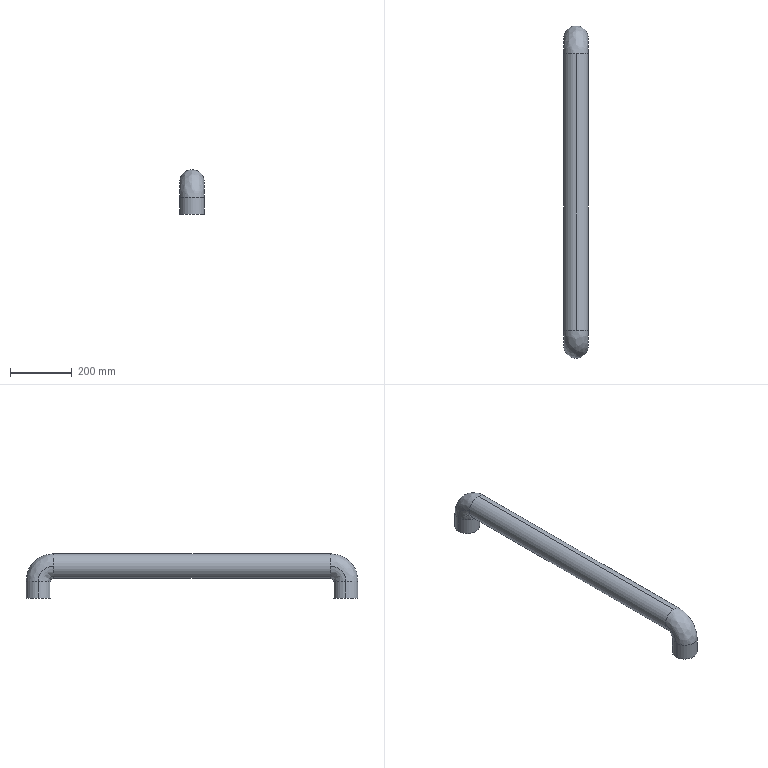Part | STEP file | Imported9 | 1 solid | 12 faces | box 80 x 1080 x 145 mm | volume 5866382 mm3 | cylinder 6 | spline 4 | plane 2 | commonest cylinder face diameters 80 x6
STEP:
#1=CARTESIAN_POINT('',(0.,0.,0.));
#2=DIRECTION('',(0.,0.,1.));
#3=DIRECTION('',(1.,0.,0.));
#4=AXIS2_PLACEMENT_3D('',#1,#2,#3);
#5=CARTESIAN_POINT('',(-920.,500.,2555.));
#6=VERTEX_POINT('',#5);
#7=CARTESIAN_POINT('',(-1000.,500.,2555.));
#8=VERTEX_POINT('',#7);
#9=CARTESIAN_POINT('',(-960.,500.,2555.));
#10=DIRECTION('',(0.,0.,1.));
#11=DIRECTION('',(-1.,0.,0.));
#12=AXIS2_PLACEMENT_3D('',#9,#10,#11);
#13=CIRCLE('',#12,40.);
#14=CARTESIAN_POINT('',(-960.,500.,2555.));
#15=DIRECTION('',(0.,0.,-1.));
#16=DIRECTION('',(-1.,0.,0.));
#17=AXIS2_PLACEMENT_3D('',#14,#15,#16);
#18=CYLINDRICAL_SURFACE('',#17,40.);
#19=CARTESIAN_POINT('',(6.283,0.));
#20=DIRECTION('',(-1.,0.));
#21=VECTOR('',#20,1.);
#22=LINE('',#19,#21);
#23=(GEOMETRIC_REPRESENTATION_CONTEXT(2)PARAMETRIC_REPRESENTATION_CONTEXT()REPRESENTATION_CONTEXT('',''));
#24=DEFINITIONAL_REPRESENTATION('',(#22),#23);
#25=PCURVE('',#18,#24);
#26=CARTESIAN_POINT('',(-1000.,500.,2555.));
#27=CARTESIAN_POINT('',(-1000.,500.,2584.289));
#28=CARTESIAN_POINT('',(-1000.,479.289,2605.));
#29=CARTESIAN_POINT('',(-1000.,450.,2605.));
#30=CARTESIAN_POINT('',(-1000.,580.,2555.));
#31=CARTESIAN_POINT('',(-1000.,580.,2631.152));
#32=CARTESIAN_POINT('',(-1000.,526.152,2685.));
#33=CARTESIAN_POINT('',(-1000.,450.,2685.));
#34=CARTESIAN_POINT('',(-920.,580.,2555.));
#35=CARTESIAN_POINT('',(-920.,580.,2631.152));
#36=CARTESIAN_POINT('',(-920.,526.152,2685.));
#37=CARTESIAN_POINT('',(-920.,450.,2685.));
#38=CARTESIAN_POINT('',(-920.,500.,2555.));
#39=CARTESIAN_POINT('',(-920.,500.,2584.289));
#40=CARTESIAN_POINT('',(-920.,479.289,2605.));
#41=CARTESIAN_POINT('',(-920.,450.,2605.));
#42=(BOUNDED_SURFACE()B_SPLINE_SURFACE(3,3,((#26,#27,#28,#29),(#30,#31,#32,#33),(#34,#35,#36,#37),(#38,#39,#40,#41)),.UNSPECIFIED.,.F.,.F.,.F.)B_SPLINE_SURFACE_WITH_KNOTS((4,4),(4,4),(0.,1.),(0.,1.),.PIECEWISE_BEZIER_KNOTS.)GEOMETRIC_REPRESENTATION_ITEM()RATIONAL_B_SPLINE_SURFACE(((1.,0.8047,0.8047,1.),(0.3333,0.2682,0.2682,0.3333),(0.3333,0.2682,0.2682,0.3333),(1.,0.8047,0.8047,1.)))REPRESENTATION_ITEM('')SURFACE());
#43=CARTESIAN_POINT('',(1.,0.));
#44=CARTESIAN_POINT('',(0.9763,0.));
#45=CARTESIAN_POINT('',(0.9319,0.));
#46=CARTESIAN_POINT('',(0.8733,0.));
#47=CARTESIAN_POINT('',(0.8206,0.));
#48=CARTESIAN_POINT('',(0.7724,0.));
#49=CARTESIAN_POINT('',(0.7279,0.));
#50=CARTESIAN_POINT('',(0.6861,0.));
#51=CARTESIAN_POINT('',(0.6465,0.));
#52=CARTESIAN_POINT('',(0.6086,0.));
#53=CARTESIAN_POINT('',(0.5718,0.));
#54=CARTESIAN_POINT('',(0.5357,0.));
#55=CARTESIAN_POINT('',(0.5,0.));
#56=CARTESIAN_POINT('',(0.4643,0.));
#57=CARTESIAN_POINT('',(0.4282,0.));
#58=CARTESIAN_POINT('',(0.3914,0.));
#59=CARTESIAN_POINT('',(0.3535,0.));
#60=CARTESIAN_POINT('',(0.3139,0.));
#61=CARTESIAN_POINT('',(0.2721,0.));
#62=CARTESIAN_POINT('',(0.2276,0.));
#63=CARTESIAN_POINT('',(0.1794,0.));
#64=CARTESIAN_POINT('',(0.1267,0.));
#65=CARTESIAN_POINT('',(0.06805,0.));
#66=CARTESIAN_POINT('',(0.02375,0.));
#67=CARTESIAN_POINT('',(0.,0.));
#68=B_SPLINE_CURVE_WITH_KNOTS('',3,(#43,#44,#45,#46,#47,#48,#49,#50,#51,#52,#53,#54,#55,#56,#57,#58,#59,#60,#61,#62,#63,#64,#65,#66,#67),.UNSPECIFIED.,.F.,.F.,(4,1,1,1,1,1,1,1,1,1,1,1,1,1,1,1,1,1,1,1,1,1,4),(3.142,3.284,3.427,3.57,3.713,3.856,3.998,4.141,4.284,4.427,4.57,4.712,4.855,4.998,5.141,5.284,5.426,5.569,5.712,5.855,5.998,6.14,6.283),.QUASI_UNIFORM_KNOTS.);
#69=(GEOMETRIC_REPRESENTATION_CONTEXT(2)PARAMETRIC_REPRESENTATION_CONTEXT()REPRESENTATION_CONTEXT('',''));
#70=DEFINITIONAL_REPRESENTATION('',(#68),#69);
#71=PCURVE('',#42,#70);
#72=SURFACE_CURVE('',#13,(#25,#71),.PCURVE_S1.);
#73=EDGE_CURVE('',#6,#8,#72,.T.);
#74=ORIENTED_EDGE('',*,*,#73,.F.);
#75=CARTESIAN_POINT('',(-920.,500.,2500.));
#76=VERTEX_POINT('',#75);
#77=CARTESIAN_POINT('',(-920.,500.,2555.));
#78=DIRECTION('',(0.,0.,-1.));
#79=VECTOR('',#78,1.);
#80=LINE('',#77,#79);
#81=CARTESIAN_POINT('',(3.142,0.));
#82=DIRECTION('',(0.,1.));
#83=VECTOR('',#82,1.);
#84=LINE('',#81,#83);
#85=(GEOMETRIC_REPRESENTATION_CONTEXT(2)PARAMETRIC_REPRESENTATION_CONTEXT()REPRESENTATION_CONTEXT('',''));
#86=DEFINITIONAL_REPRESENTATION('',(#84),#85);
#87=PCURVE('',#18,#86);
#88=CARTESIAN_POINT('',(-960.,500.,2555.));
#89=DIRECTION('',(0.,0.,-1.));
#90=DIRECTION('',(-1.,0.,0.));
#91=AXIS2_PLACEMENT_3D('',#88,#89,#90);
#92=CYLINDRICAL_SURFACE('',#91,40.);
#93=CARTESIAN_POINT('',(3.142,0.));
#94=DIRECTION('',(0.,1.));
#95=VECTOR('',#94,1.);
#96=LINE('',#93,#95);
#97=(GEOMETRIC_REPRESENTATION_CONTEXT(2)PARAMETRIC_REPRESENTATION_CONTEXT()REPRESENTATION_CONTEXT('',''));
#98=DEFINITIONAL_REPRESENTATION('',(#96),#97);
#99=PCURVE('',#92,#98);
#100=SURFACE_CURVE('',#80,(#87,#99),.PCURVE_S1.);
#101=EDGE_CURVE('',#6,#76,#100,.T.);
#102=ORIENTED_EDGE('',*,*,#101,.T.);
#103=CARTESIAN_POINT('',(-1000.,500.,2500.));
#104=VERTEX_POINT('',#103);
#105=CARTESIAN_POINT('',(-960.,500.,2500.));
#106=DIRECTION('',(0.,0.,-1.));
#107=DIRECTION('',(-1.,0.,0.));
#108=AXIS2_PLACEMENT_3D('',#105,#106,#107);
#109=CIRCLE('',#108,40.);
#110=CARTESIAN_POINT('',(0.,55.));
#111=DIRECTION('',(1.,0.));
#112=VECTOR('',#111,1.);
#113=LINE('',#110,#112);
#114=(GEOMETRIC_REPRESENTATION_CONTEXT(2)PARAMETRIC_REPRESENTATION_CONTEXT()REPRESENTATION_CONTEXT('',''));
#115=DEFINITIONAL_REPRESENTATION('',(#113),#114);
#116=PCURVE('',#18,#115);
#117=CARTESIAN_POINT('',(0.,0.,2500.));
#118=DIRECTION('',(0.,0.,-1.));
#119=DIRECTION('',(-1.,0.,0.));
#120=AXIS2_PLACEMENT_3D('',#117,#118,#119);
#121=PLANE('',#120);
#122=CARTESIAN_POINT('',(960.,500.));
#123=DIRECTION('',(1.,0.));
#124=AXIS2_PLACEMENT_2D('',#122,#123);
#125=CIRCLE('',#124,40.);
#126=(GEOMETRIC_REPRESENTATION_CONTEXT(2)PARAMETRIC_REPRESENTATION_CONTEXT()REPRESENTATION_CONTEXT('',''));
#127=DEFINITIONAL_REPRESENTATION('',(#125),#126);
#128=PCURVE('',#121,#127);
#129=SURFACE_CURVE('',#109,(#116,#128),.PCURVE_S1.);
#130=EDGE_CURVE('',#104,#76,#129,.T.);
#131=ORIENTED_EDGE('',*,*,#130,.F.);
#132=CARTESIAN_POINT('',(-1000.,500.,2555.));
#133=DIRECTION('',(0.,0.,-1.));
#134=VECTOR('',#133,1.);
#135=LINE('',#132,#134);
#136=CARTESIAN_POINT('',(0.,0.));
#137=DIRECTION('',(0.,1.));
#138=VECTOR('',#137,1.);
#139=LINE('',#136,#138);
#140=(GEOMETRIC_REPRESENTATION_CONTEXT(2)PARAMETRIC_REPRESENTATION_CONTEXT()REPRESENTATION_CONTEXT('',''));
#141=DEFINITIONAL_REPRESENTATION('',(#139),#140);
#142=PCURVE('',#18,#141);
#143=CARTESIAN_POINT('',(6.283,0.));
#144=DIRECTION('',(0.,1.));
#145=VECTOR('',#144,1.);
#146=LINE('',#143,#145);
#147=(GEOMETRIC_REPRESENTATION_CONTEXT(2)PARAMETRIC_REPRESENTATION_CONTEXT()REPRESENTATION_CONTEXT('',''));
#148=DEFINITIONAL_REPRESENTATION('',(#146),#147);
#149=PCURVE('',#92,#148);
#150=SURFACE_CURVE('',#135,(#142,#149),.PCURVE_S1.);
#151=EDGE_CURVE('',#8,#104,#150,.T.);
#152=ORIENTED_EDGE('',*,*,#151,.F.);
#153=EDGE_LOOP('',(#74,#102,#131,#152));
#154=FACE_BOUND('',#153,.T.);
#155=ADVANCED_FACE('',(#154),#18,.T.);
#156=CARTESIAN_POINT('',(-920.,450.,2605.));
#157=VERTEX_POINT('',#156);
#158=CARTESIAN_POINT('',(-960.,450.,2645.));
#159=VERTEX_POINT('',#158);
#160=CARTESIAN_POINT('',(-960.,450.,2605.));
#161=DIRECTION('',(0.,-1.,0.));
#162=DIRECTION('',(0.,0.,-1.));
#163=AXIS2_PLACEMENT_3D('',#160,#161,#162);
#164=CIRCLE('',#163,40.);
#165=CARTESIAN_POINT('',(-960.,450.,2605.));
#166=DIRECTION('',(0.,-1.,0.));
#167=DIRECTION('',(0.,0.,-1.));
#168=AXIS2_PLACEMENT_3D('',#165,#166,#167);
#169=CYLINDRICAL_SURFACE('',#168,40.);
#170=CARTESIAN_POINT('',(0.,0.));
#171=DIRECTION('',(1.,0.));
#172=VECTOR('',#171,1.);
#173=LINE('',#170,#172);
#174=(GEOMETRIC_REPRESENTATION_CONTEXT(2)PARAMETRIC_REPRESENTATION_CONTEXT()REPRESENTATION_CONTEXT('',''));
#175=DEFINITIONAL_REPRESENTATION('',(#173),#174);
#176=PCURVE('',#169,#175);
#177=CARTESIAN_POINT('',(1.,1.));
#178=CARTESIAN_POINT('',(0.9881,1.));
#179=CARTESIAN_POINT('',(0.9651,1.));
#180=CARTESIAN_POINT('',(0.9329,1.));
#181=CARTESIAN_POINT('',(0.9026,1.));
#182=CARTESIAN_POINT('',(0.874,1.));
#183=CARTESIAN_POINT('',(0.8469,1.));
#184=CARTESIAN_POINT('',(0.8211,1.));
#185=CARTESIAN_POINT('',(0.7965,1.));
#186=CARTESIAN_POINT('',(0.7729,1.));
#187=CARTESIAN_POINT('',(0.7501,1.));
#188=CARTESIAN_POINT('',(0.7282,1.));
#189=CARTESIAN_POINT('',(0.707,1.));
#190=CARTESIAN_POINT('',(0.6864,1.));
#191=CARTESIAN_POINT('',(0.6663,1.));
#192=CARTESIAN_POINT('',(0.6467,1.));
#193=CARTESIAN_POINT('',(0.6276,1.));
#194=CARTESIAN_POINT('',(0.6087,1.));
#195=CARTESIAN_POINT('',(0.5902,1.));
#196=CARTESIAN_POINT('',(0.5719,1.));
#197=CARTESIAN_POINT('',(0.5537,1.));
#198=CARTESIAN_POINT('',(0.5357,1.));
#199=CARTESIAN_POINT('',(0.5178,1.));
#200=CARTESIAN_POINT('',(0.506,1.));
#201=CARTESIAN_POINT('',(0.5,1.));
#202=B_SPLINE_CURVE_WITH_KNOTS('',3,(#177,#178,#179,#180,#181,#182,#183,#184,#185,#186,#187,#188,#189,#190,#191,#192,#193,#194,#195,#196,#197,#198,#199,#200,#201),.UNSPECIFIED.,.F.,.F.,(4,1,1,1,1,1,1,1,1,1,1,1,1,1,1,1,1,1,1,1,1,1,4),(1.571,1.642,1.714,1.785,1.856,1.928,1.999,2.071,2.142,2.213,2.285,2.356,2.428,2.499,2.57,2.642,2.713,2.785,2.856,2.927,2.999,3.07,3.142),.QUASI_UNIFORM_KNOTS.);
#203=(GEOMETRIC_REPRESENTATION_CONTEXT(2)PARAMETRIC_REPRESENTATION_CONTEXT()REPRESENTATION_CONTEXT('',''));
#204=DEFINITIONAL_REPRESENTATION('',(#202),#203);
#205=PCURVE('',#42,#204);
#206=SURFACE_CURVE('',#164,(#176,#205),.PCURVE_S1.);
#207=EDGE_CURVE('',#157,#159,#206,.T.);
#208=ORIENTED_EDGE('',*,*,#207,.T.);
#209=CARTESIAN_POINT('',(-960.,-450.,2645.));
#210=VERTEX_POINT('',#209);
#211=CARTESIAN_POINT('',(-960.,450.,2645.));
#212=DIRECTION('',(0.,-1.,0.));
#213=VECTOR('',#212,1.);
#214=LINE('',#211,#213);
#215=CARTESIAN_POINT('',(3.142,0.));
#216=DIRECTION('',(0.,1.));
#217=VECTOR('',#216,1.);
#218=LINE('',#215,#217);
#219=(GEOMETRIC_REPRESENTATION_CONTEXT(2)PARAMETRIC_REPRESENTATION_CONTEXT()REPRESENTATION_CONTEXT('',''));
#220=DEFINITIONAL_REPRESENTATION('',(#218),#219);
#221=PCURVE('',#169,#220);
#222=CARTESIAN_POINT('',(-960.,450.,2605.));
#223=DIRECTION('',(0.,-1.,0.));
#224=DIRECTION('',(0.,0.,-1.));
#225=AXIS2_PLACEMENT_3D('',#222,#223,#224);
#226=CYLINDRICAL_SURFACE('',#225,40.);
#227=CARTESIAN_POINT('',(3.142,0.));
#228=DIRECTION('',(0.,1.));
#229=VECTOR('',#228,1.);
#230=LINE('',#227,#229);
#231=(GEOMETRIC_REPRESENTATION_CONTEXT(2)PARAMETRIC_REPRESENTATION_CONTEXT()REPRESENTATION_CONTEXT('',''));
#232=DEFINITIONAL_REPRESENTATION('',(#230),#231);
#233=PCURVE('',#226,#232);
#234=SURFACE_CURVE('',#214,(#221,#233),.PCURVE_S1.);
#235=EDGE_CURVE('',#159,#210,#234,.T.);
#236=ORIENTED_EDGE('',*,*,#235,.T.);
#237=CARTESIAN_POINT('',(-920.,-450.,2605.));
#238=VERTEX_POINT('',#237);
#239=CARTESIAN_POINT('',(-960.,-450.,2605.));
#240=DIRECTION('',(0.,-1.,0.));
#241=DIRECTION('',(1.,0.,0.));
#242=AXIS2_PLACEMENT_3D('',#239,#240,#241);
#243=CIRCLE('',#242,40.);
#244=CARTESIAN_POINT('',(1.571,900.));
#245=DIRECTION('',(1.,0.));
#246=VECTOR('',#245,1.);
#247=LINE('',#244,#246);
#248=(GEOMETRIC_REPRESENTATION_CONTEXT(2)PARAMETRIC_REPRESENTATION_CONTEXT()REPRESENTATION_CONTEXT('',''));
#249=DEFINITIONAL_REPRESENTATION('',(#247),#248);
#250=PCURVE('',#169,#249);
#251=CARTESIAN_POINT('',(-1000.,-450.,2605.));
#252=CARTESIAN_POINT('',(-1000.,-479.289,2605.));
#253=CARTESIAN_POINT('',(-1000.,-500.,2584.289));
#254=CARTESIAN_POINT('',(-1000.,-500.,2555.));
#255=CARTESIAN_POINT('',(-1000.,-450.,2685.));
#256=CARTESIAN_POINT('',(-1000.,-526.152,2685.));
#257=CARTESIAN_POINT('',(-1000.,-580.,2631.152));
#258=CARTESIAN_POINT('',(-1000.,-580.,2555.));
#259=CARTESIAN_POINT('',(-920.,-450.,2685.));
#260=CARTESIAN_POINT('',(-920.,-526.152,2685.));
#261=CARTESIAN_POINT('',(-920.,-580.,2631.152));
#262=CARTESIAN_POINT('',(-920.,-580.,2555.));
#263=CARTESIAN_POINT('',(-920.,-450.,2605.));
#264=CARTESIAN_POINT('',(-920.,-479.289,2605.));
#265=CARTESIAN_POINT('',(-920.,-500.,2584.289));
#266=CARTESIAN_POINT('',(-920.,-500.,2555.));
#267=(BOUNDED_SURFACE()B_SPLINE_SURFACE(3,3,((#251,#252,#253,#254),(#255,#256,#257,#258),(#259,#260,#261,#262),(#263,#264,#265,#266)),.UNSPECIFIED.,.F.,.F.,.F.)B_SPLINE_SURFACE_WITH_KNOTS((4,4),(4,4),(0.,1.),(0.,1.),.PIECEWISE_BEZIER_KNOTS.)GEOMETRIC_REPRESENTATION_ITEM()RATIONAL_B_SPLINE_SURFACE(((1.,0.8047,0.8047,1.),(0.3333,0.2682,0.2682,0.3333),(0.3333,0.2682,0.2682,0.3333),(1.,0.8047,0.8047,1.)))REPRESENTATION_ITEM('')SURFACE());
#268=CARTESIAN_POINT('',(1.,0.));
#269=CARTESIAN_POINT('',(0.9881,0.));
#270=CARTESIAN_POINT('',(0.9651,0.));
#271=CARTESIAN_POINT('',(0.9329,0.));
#272=CARTESIAN_POINT('',(0.9026,0.));
#273=CARTESIAN_POINT('',(0.874,0.));
#274=CARTESIAN_POINT('',(0.8469,0.));
#275=CARTESIAN_POINT('',(0.8211,0.));
#276=CARTESIAN_POINT('',(0.7965,0.));
#277=CARTESIAN_POINT('',(0.7729,0.));
#278=CARTESIAN_POINT('',(0.7501,0.));
#279=CARTESIAN_POINT('',(0.7282,0.));
#280=CARTESIAN_POINT('',(0.707,0.));
#281=CARTESIAN_POINT('',(0.6864,0.));
#282=CARTESIAN_POINT('',(0.6663,0.));
#283=CARTESIAN_POINT('',(0.6467,0.));
#284=CARTESIAN_POINT('',(0.6276,0.));
#285=CARTESIAN_POINT('',(0.6087,0.));
#286=CARTESIAN_POINT('',(0.5902,0.));
#287=CARTESIAN_POINT('',(0.5719,0.));
#288=CARTESIAN_POINT('',(0.5537,0.));
#289=CARTESIAN_POINT('',(0.5357,0.));
#290=CARTESIAN_POINT('',(0.5178,0.));
#291=CARTESIAN_POINT('',(0.506,0.));
#292=CARTESIAN_POINT('',(0.5,0.));
#293=B_SPLINE_CURVE_WITH_KNOTS('',3,(#268,#269,#270,#271,#272,#273,#274,#275,#276,#277,#278,#279,#280,#281,#282,#283,#284,#285,#286,#287,#288,#289,#290,#291,#292),.UNSPECIFIED.,.F.,.F.,(4,1,1,1,1,1,1,1,1,1,1,1,1,1,1,1,1,1,1,1,1,1,4),(0.,0.0714,0.1428,0.2142,0.2856,0.357,0.4284,0.4998,0.5712,0.6426,0.714,0.7854,0.8568,0.9282,0.9996,1.071,1.142,1.214,1.285,1.357,1.428,1.499,1.571),.QUASI_UNIFORM_KNOTS.);
#294=(GEOMETRIC_REPRESENTATION_CONTEXT(2)PARAMETRIC_REPRESENTATION_CONTEXT()REPRESENTATION_CONTEXT('',''));
#295=DEFINITIONAL_REPRESENTATION('',(#293),#294);
#296=PCURVE('',#267,#295);
#297=SURFACE_CURVE('',#243,(#250,#296),.PCURVE_S1.);
#298=EDGE_CURVE('',#238,#210,#297,.T.);
#299=ORIENTED_EDGE('',*,*,#298,.F.);
#300=CARTESIAN_POINT('',(-960.,-450.,2565.));
#301=VERTEX_POINT('',#300);
#302=CARTESIAN_POINT('',(-960.,-450.,2605.));
#303=DIRECTION('',(0.,-1.,0.));
#304=DIRECTION('',(-1.,0.,0.));
#305=AXIS2_PLACEMENT_3D('',#302,#303,#304);
#306=CIRCLE('',#305,40.);
#307=CARTESIAN_POINT('',(-1.571,900.));
#308=DIRECTION('',(1.,0.));
#309=VECTOR('',#308,1.);
#310=LINE('',#307,#309);
#311=(GEOMETRIC_REPRESENTATION_CONTEXT(2)PARAMETRIC_REPRESENTATION_CONTEXT()REPRESENTATION_CONTEXT('',''));
#312=DEFINITIONAL_REPRESENTATION('',(#310),#311);
#313=PCURVE('',#169,#312);
#314=CARTESIAN_POINT('',(-920.,-450.,2605.));
#315=CARTESIAN_POINT('',(-920.,-479.289,2605.));
#316=CARTESIAN_POINT('',(-920.,-500.,2584.289));
#317=CARTESIAN_POINT('',(-920.,-500.,2555.));
#318=CARTESIAN_POINT('',(-920.,-450.,2525.));
#319=CARTESIAN_POINT('',(-920.,-432.426,2525.));
#320=CARTESIAN_POINT('',(-920.,-420.,2537.426));
#321=CARTESIAN_POINT('',(-920.,-420.,2555.));
#322=CARTESIAN_POINT('',(-1000.,-450.,2525.));
#323=CARTESIAN_POINT('',(-1000.,-432.426,2525.));
#324=CARTESIAN_POINT('',(-1000.,-420.,2537.426));
#325=CARTESIAN_POINT('',(-1000.,-420.,2555.));
#326=CARTESIAN_POINT('',(-1000.,-450.,2605.));
#327=CARTESIAN_POINT('',(-1000.,-479.289,2605.));
#328=CARTESIAN_POINT('',(-1000.,-500.,2584.289));
#329=CARTESIAN_POINT('',(-1000.,-500.,2555.));
#330=(BOUNDED_SURFACE()B_SPLINE_SURFACE(3,3,((#314,#315,#316,#317),(#318,#319,#320,#321),(#322,#323,#324,#325),(#326,#327,#328,#329)),.UNSPECIFIED.,.F.,.F.,.F.)B_SPLINE_SURFACE_WITH_KNOTS((4,4),(4,4),(0.,1.),(0.,1.),.PIECEWISE_BEZIER_KNOTS.)GEOMETRIC_REPRESENTATION_ITEM()RATIONAL_B_SPLINE_SURFACE(((1.,0.8047,0.8047,1.),(0.3333,0.2682,0.2682,0.3333),(0.3333,0.2682,0.2682,0.3333),(1.,0.8047,0.8047,1.)))REPRESENTATION_ITEM('')SURFACE());
#331=CARTESIAN_POINT('',(0.5,0.));
#332=CARTESIAN_POINT('',(0.494,0.));
#333=CARTESIAN_POINT('',(0.4822,0.));
#334=CARTESIAN_POINT('',(0.4643,0.));
#335=CARTESIAN_POINT('',(0.4463,0.));
#336=CARTESIAN_POINT('',(0.4281,0.));
#337=CARTESIAN_POINT('',(0.4098,0.));
#338=CARTESIAN_POINT('',(0.3913,0.));
#339=CARTESIAN_POINT('',(0.3724,0.));
#340=CARTESIAN_POINT('',(0.3533,0.));
#341=CARTESIAN_POINT('',(0.3337,0.));
#342=CARTESIAN_POINT('',(0.3136,0.));
#343=CARTESIAN_POINT('',(0.293,0.));
#344=CARTESIAN_POINT('',(0.2718,0.));
#345=CARTESIAN_POINT('',(0.2499,0.));
#346=CARTESIAN_POINT('',(0.2271,0.));
#347=CARTESIAN_POINT('',(0.2035,0.));
#348=CARTESIAN_POINT('',(0.1789,0.));
#349=CARTESIAN_POINT('',(0.1531,0.));
#350=CARTESIAN_POINT('',(0.126,0.));
#351=CARTESIAN_POINT('',(0.09736,0.));
#352=CARTESIAN_POINT('',(0.06707,0.));
#353=CARTESIAN_POINT('',(0.03485,0.));
#354=CARTESIAN_POINT('',(0.0119,0.));
#355=CARTESIAN_POINT('',(0.,0.));
#356=B_SPLINE_CURVE_WITH_KNOTS('',3,(#331,#332,#333,#334,#335,#336,#337,#338,#339,#340,#341,#342,#343,#344,#345,#346,#347,#348,#349,#350,#351,#352,#353,#354,#355),.UNSPECIFIED.,.F.,.F.,(4,1,1,1,1,1,1,1,1,1,1,1,1,1,1,1,1,1,1,1,1,1,4),(1.571,1.642,1.714,1.785,1.856,1.928,1.999,2.071,2.142,2.213,2.285,2.356,2.428,2.499,2.57,2.642,2.713,2.785,2.856,2.927,2.999,3.07,3.142),.QUASI_UNIFORM_KNOTS.);
#357=(GEOMETRIC_REPRESENTATION_CONTEXT(2)PARAMETRIC_REPRESENTATION_CONTEXT()REPRESENTATION_CONTEXT('',''));
#358=DEFINITIONAL_REPRESENTATION('',(#356),#357);
#359=PCURVE('',#330,#358);
#360=SURFACE_CURVE('',#306,(#313,#359),.PCURVE_S1.);
#361=EDGE_CURVE('',#301,#238,#360,.T.);
#362=ORIENTED_EDGE('',*,*,#361,.F.);
#363=CARTESIAN_POINT('',(-960.,450.,2565.));
#364=VERTEX_POINT('',#363);
#365=CARTESIAN_POINT('',(-960.,450.,2565.));
#366=DIRECTION('',(0.,-1.,0.));
#367=VECTOR('',#366,1.);
#368=LINE('',#365,#367);
#369=CARTESIAN_POINT('',(0.,0.));
#370=DIRECTION('',(0.,1.));
#371=VECTOR('',#370,1.);
#372=LINE('',#369,#371);
#373=(GEOMETRIC_REPRESENTATION_CONTEXT(2)PARAMETRIC_REPRESENTATION_CONTEXT()REPRESENTATION_CONTEXT('',''));
#374=DEFINITIONAL_REPRESENTATION('',(#372),#373);
#375=PCURVE('',#169,#374);
#376=CARTESIAN_POINT('',(6.283,0.));
#377=DIRECTION('',(0.,1.));
#378=VECTOR('',#377,1.);
#379=LINE('',#376,#378);
#380=(GEOMETRIC_REPRESENTATION_CONTEXT(2)PARAMETRIC_REPRESENTATION_CONTEXT()REPRESENTATION_CONTEXT('',''));
#381=DEFINITIONAL_REPRESENTATION('',(#379),#380);
#382=PCURVE('',#226,#381);
#383=SURFACE_CURVE('',#368,(#375,#382),.PCURVE_S1.);
#384=EDGE_CURVE('',#364,#301,#383,.T.);
#385=ORIENTED_EDGE('',*,*,#384,.F.);
#386=CARTESIAN_POINT('',(-960.,450.,2605.));
#387=DIRECTION('',(0.,-1.,0.));
#388=DIRECTION('',(0.,0.,-1.));
#389=AXIS2_PLACEMENT_3D('',#386,#387,#388);
#390=CIRCLE('',#389,40.);
#391=CARTESIAN_POINT('',(0.,0.));
#392=DIRECTION('',(1.,0.));
#393=VECTOR('',#392,1.);
#394=LINE('',#391,#393);
#395=(GEOMETRIC_REPRESENTATION_CONTEXT(2)PARAMETRIC_REPRESENTATION_CONTEXT()REPRESENTATION_CONTEXT('',''));
#396=DEFINITIONAL_REPRESENTATION('',(#394),#395);
#397=PCURVE('',#169,#396);
#398=CARTESIAN_POINT('',(-920.,500.,2555.));
#399=CARTESIAN_POINT('',(-920.,500.,2584.289));
#400=CARTESIAN_POINT('',(-920.,479.289,2605.));
#401=CARTESIAN_POINT('',(-920.,450.,2605.));
#402=CARTESIAN_POINT('',(-920.,420.,2555.));
#403=CARTESIAN_POINT('',(-920.,420.,2537.426));
#404=CARTESIAN_POINT('',(-920.,432.426,2525.));
#405=CARTESIAN_POINT('',(-920.,450.,2525.));
#406=CARTESIAN_POINT('',(-1000.,420.,2555.));
#407=CARTESIAN_POINT('',(-1000.,420.,2537.426));
#408=CARTESIAN_POINT('',(-1000.,432.426,2525.));
#409=CARTESIAN_POINT('',(-1000.,450.,2525.));
#410=CARTESIAN_POINT('',(-1000.,500.,2555.));
#411=CARTESIAN_POINT('',(-1000.,500.,2584.289));
#412=CARTESIAN_POINT('',(-1000.,479.289,2605.));
#413=CARTESIAN_POINT('',(-1000.,450.,2605.));
#414=(BOUNDED_SURFACE()B_SPLINE_SURFACE(3,3,((#398,#399,#400,#401),(#402,#403,#404,#405),(#406,#407,#408,#409),(#410,#411,#412,#413)),.UNSPECIFIED.,.F.,.F.,.F.)B_SPLINE_SURFACE_WITH_KNOTS((4,4),(4,4),(0.,1.),(0.,1.),.PIECEWISE_BEZIER_KNOTS.)GEOMETRIC_REPRESENTATION_ITEM()RATIONAL_B_SPLINE_SURFACE(((1.,0.8047,0.8047,1.),(0.3333,0.2682,0.2682,0.3333),(0.3333,0.2682,0.2682,0.3333),(1.,0.8047,0.8047,1.)))REPRESENTATION_ITEM('')SURFACE());
#415=CARTESIAN_POINT('',(0.5,1.));
#416=CARTESIAN_POINT('',(0.494,1.));
#417=CARTESIAN_POINT('',(0.4822,1.));
#418=CARTESIAN_POINT('',(0.4643,1.));
#419=CARTESIAN_POINT('',(0.4463,1.));
#420=CARTESIAN_POINT('',(0.4281,1.));
#421=CARTESIAN_POINT('',(0.4098,1.));
#422=CARTESIAN_POINT('',(0.3913,1.));
#423=CARTESIAN_POINT('',(0.3724,1.));
#424=CARTESIAN_POINT('',(0.3533,1.));
#425=CARTESIAN_POINT('',(0.3337,1.));
#426=CARTESIAN_POINT('',(0.3136,1.));
#427=CARTESIAN_POINT('',(0.293,1.));
#428=CARTESIAN_POINT('',(0.2718,1.));
#429=CARTESIAN_POINT('',(0.2499,1.));
#430=CARTESIAN_POINT('',(0.2271,1.));
#431=CARTESIAN_POINT('',(0.2035,1.));
#432=CARTESIAN_POINT('',(0.1789,1.));
#433=CARTESIAN_POINT('',(0.1531,1.));
#434=CARTESIAN_POINT('',(0.126,1.));
#435=CARTESIAN_POINT('',(0.09736,1.));
#436=CARTESIAN_POINT('',(0.06707,1.));
#437=CARTESIAN_POINT('',(0.03485,1.));
#438=CARTESIAN_POINT('',(0.0119,1.));
#439=CARTESIAN_POINT('',(0.,1.));
#440=B_SPLINE_CURVE_WITH_KNOTS('',3,(#415,#416,#417,#418,#419,#420,#421,#422,#423,#424,#425,#426,#427,#428,#429,#430,#431,#432,#433,#434,#435,#436,#437,#438,#439),.UNSPECIFIED.,.F.,.F.,(4,1,1,1,1,1,1,1,1,1,1,1,1,1,1,1,1,1,1,1,1,1,4),(0.,0.0714,0.1428,0.2142,0.2856,0.357,0.4284,0.4998,0.5712,0.6426,0.714,0.7854,0.8568,0.9282,0.9996,1.071,1.142,1.214,1.285,1.357,1.428,1.499,1.571),.QUASI_UNIFORM_KNOTS.);
#441=(GEOMETRIC_REPRESENTATION_CONTEXT(2)PARAMETRIC_REPRESENTATION_CONTEXT()REPRESENTATION_CONTEXT('',''));
#442=DEFINITIONAL_REPRESENTATION('',(#440),#441);
#443=PCURVE('',#414,#442);
#444=SURFACE_CURVE('',#390,(#397,#443),.PCURVE_S1.);
#445=EDGE_CURVE('',#364,#157,#444,.T.);
#446=ORIENTED_EDGE('',*,*,#445,.T.);
#447=EDGE_LOOP('',(#208,#236,#299,#362,#385,#446));
#448=FACE_BOUND('',#447,.T.);
#449=ADVANCED_FACE('',(#448),#169,.T.);
#450=CARTESIAN_POINT('',(-1000.,-500.,2555.));
#451=VERTEX_POINT('',#450);
#452=CARTESIAN_POINT('',(-920.,-500.,2555.));
#453=VERTEX_POINT('',#452);
#454=CARTESIAN_POINT('',(-960.,-500.,2555.));
#455=DIRECTION('',(0.,0.,-1.));
#456=DIRECTION('',(0.,1.,0.));
#457=AXIS2_PLACEMENT_3D('',#454,#455,#456);
#458=CIRCLE('',#457,40.);
#459=CARTESIAN_POINT('',(-960.,-500.,2555.));
#460=DIRECTION('',(0.,0.,-1.));
#461=DIRECTION('',(-1.,0.,0.));
#462=AXIS2_PLACEMENT_3D('',#459,#460,#461);
#463=CYLINDRICAL_SURFACE('',#462,40.);
#464=CARTESIAN_POINT('',(-4.712,0.));
#465=DIRECTION('',(1.,0.));
#466=VECTOR('',#465,1.);
#467=LINE('',#464,#466);
#468=(GEOMETRIC_REPRESENTATION_CONTEXT(2)PARAMETRIC_REPRESENTATION_CONTEXT()REPRESENTATION_CONTEXT('',''));
#469=DEFINITIONAL_REPRESENTATION('',(#467),#468);
#470=PCURVE('',#463,#469);
#471=CARTESIAN_POINT('',(1.,1.));
#472=CARTESIAN_POINT('',(0.9763,1.));
#473=CARTESIAN_POINT('',(0.9319,1.));
#474=CARTESIAN_POINT('',(0.8733,1.));
#475=CARTESIAN_POINT('',(0.8206,1.));
#476=CARTESIAN_POINT('',(0.7724,1.));
#477=CARTESIAN_POINT('',(0.7279,1.));
#478=CARTESIAN_POINT('',(0.6861,1.));
#479=CARTESIAN_POINT('',(0.6465,1.));
#480=CARTESIAN_POINT('',(0.6086,1.));
#481=CARTESIAN_POINT('',(0.5718,1.));
#482=CARTESIAN_POINT('',(0.5357,1.));
#483=CARTESIAN_POINT('',(0.5,1.));
#484=CARTESIAN_POINT('',(0.4643,1.));
#485=CARTESIAN_POINT('',(0.4282,1.));
#486=CARTESIAN_POINT('',(0.3914,1.));
#487=CARTESIAN_POINT('',(0.3535,1.));
#488=CARTESIAN_POINT('',(0.3139,1.));
#489=CARTESIAN_POINT('',(0.2721,1.));
#490=CARTESIAN_POINT('',(0.2276,1.));
#491=CARTESIAN_POINT('',(0.1794,1.));
#492=CARTESIAN_POINT('',(0.1267,1.));
#493=CARTESIAN_POINT('',(0.06805,1.));
#494=CARTESIAN_POINT('',(0.02375,1.));
#495=CARTESIAN_POINT('',(0.,1.));
#496=B_SPLINE_CURVE_WITH_KNOTS('',3,(#471,#472,#473,#474,#475,#476,#477,#478,#479,#480,#481,#482,#483,#484,#485,#486,#487,#488,#489,#490,#491,#492,#493,#494,#495),.UNSPECIFIED.,.F.,.F.,(4,1,1,1,1,1,1,1,1,1,1,1,1,1,1,1,1,1,1,1,1,1,4),(4.712,4.855,4.998,5.141,5.284,5.426,5.569,5.712,5.855,5.998,6.14,6.283,6.426,6.569,6.712,6.854,6.997,7.14,7.283,7.426,7.568,7.711,7.854),.QUASI_UNIFORM_KNOTS.);
#497=(GEOMETRIC_REPRESENTATION_CONTEXT(2)PARAMETRIC_REPRESENTATION_CONTEXT()REPRESENTATION_CONTEXT('',''));
#498=DEFINITIONAL_REPRESENTATION('',(#496),#497);
#499=PCURVE('',#330,#498);
#500=SURFACE_CURVE('',#458,(#470,#499),.PCURVE_S1.);
#501=EDGE_CURVE('',#451,#453,#500,.T.);
#502=ORIENTED_EDGE('',*,*,#501,.T.);
#503=CARTESIAN_POINT('',(-920.,-500.,2500.));
#504=VERTEX_POINT('',#503);
#505=CARTESIAN_POINT('',(-920.,-500.,2555.));
#506=DIRECTION('',(0.,0.,-1.));
#507=VECTOR('',#506,1.);
#508=LINE('',#505,#507);
#509=CARTESIAN_POINT('',(3.142,0.));
#510=DIRECTION('',(0.,1.));
#511=VECTOR('',#510,1.);
#512=LINE('',#509,#511);
#513=(GEOMETRIC_REPRESENTATION_CONTEXT(2)PARAMETRIC_REPRESENTATION_CONTEXT()REPRESENTATION_CONTEXT('',''));
#514=DEFINITIONAL_REPRESENTATION('',(#512),#513);
#515=PCURVE('',#463,#514);
#516=CARTESIAN_POINT('',(-960.,-500.,2555.));
#517=DIRECTION('',(0.,0.,-1.));
#518=DIRECTION('',(-1.,0.,0.));
#519=AXIS2_PLACEMENT_3D('',#516,#517,#518);
#520=CYLINDRICAL_SURFACE('',#519,40.);
#521=CARTESIAN_POINT('',(3.142,0.));
#522=DIRECTION('',(0.,1.));
#523=VECTOR('',#522,1.);
#524=LINE('',#521,#523);
#525=(GEOMETRIC_REPRESENTATION_CONTEXT(2)PARAMETRIC_REPRESENTATION_CONTEXT()REPRESENTATION_CONTEXT('',''));
#526=DEFINITIONAL_REPRESENTATION('',(#524),#525);
#527=PCURVE('',#520,#526);
#528=SURFACE_CURVE('',#508,(#515,#527),.PCURVE_S1.);
#529=EDGE_CURVE('',#453,#504,#528,.T.);
#530=ORIENTED_EDGE('',*,*,#529,.T.);
#531=CARTESIAN_POINT('',(-1000.,-500.,2500.));
#532=VERTEX_POINT('',#531);
#533=CARTESIAN_POINT('',(-960.,-500.,2500.));
#534=DIRECTION('',(0.,0.,-1.));
#535=DIRECTION('',(-1.,0.,0.));
#536=AXIS2_PLACEMENT_3D('',#533,#534,#535);
#537=CIRCLE('',#536,40.);
#538=CARTESIAN_POINT('',(0.,55.));
#539=DIRECTION('',(1.,0.));
#540=VECTOR('',#539,1.);
#541=LINE('',#538,#540);
#542=(GEOMETRIC_REPRESENTATION_CONTEXT(2)PARAMETRIC_REPRESENTATION_CONTEXT()REPRESENTATION_CONTEXT('',''));
#543=DEFINITIONAL_REPRESENTATION('',(#541),#542);
#544=PCURVE('',#463,#543);
#545=CARTESIAN_POINT('',(0.,0.,2500.));
#546=DIRECTION('',(0.,0.,-1.));
#547=DIRECTION('',(-1.,0.,0.));
#548=AXIS2_PLACEMENT_3D('',#545,#546,#547);
#549=PLANE('',#548);
#550=CARTESIAN_POINT('',(960.,-500.));
#551=DIRECTION('',(1.,0.));
#552=AXIS2_PLACEMENT_2D('',#550,#551);
#553=CIRCLE('',#552,40.);
#554=(GEOMETRIC_REPRESENTATION_CONTEXT(2)PARAMETRIC_REPRESENTATION_CONTEXT()REPRESENTATION_CONTEXT('',''));
#555=DEFINITIONAL_REPRESENTATION('',(#553),#554);
#556=PCURVE('',#549,#555);
#557=SURFACE_CURVE('',#537,(#544,#556),.PCURVE_S1.);
#558=EDGE_CURVE('',#532,#504,#557,.T.);
#559=ORIENTED_EDGE('',*,*,#558,.F.);
#560=CARTESIAN_POINT('',(-1000.,-500.,2555.));
#561=DIRECTION('',(0.,0.,-1.));
#562=VECTOR('',#561,1.);
#563=LINE('',#560,#562);
#564=CARTESIAN_POINT('',(0.,0.));
#565=DIRECTION('',(0.,1.));
#566=VECTOR('',#565,1.);
#567=LINE('',#564,#566);
#568=(GEOMETRIC_REPRESENTATION_CONTEXT(2)PARAMETRIC_REPRESENTATION_CONTEXT()REPRESENTATION_CONTEXT('',''));
#569=DEFINITIONAL_REPRESENTATION('',(#567),#568);
#570=PCURVE('',#463,#569);
#571=CARTESIAN_POINT('',(6.283,0.));
#572=DIRECTION('',(0.,1.));
#573=VECTOR('',#572,1.);
#574=LINE('',#571,#573);
#575=(GEOMETRIC_REPRESENTATION_CONTEXT(2)PARAMETRIC_REPRESENTATION_CONTEXT()REPRESENTATION_CONTEXT('',''));
#576=DEFINITIONAL_REPRESENTATION('',(#574),#575);
#577=PCURVE('',#520,#576);
#578=SURFACE_CURVE('',#563,(#570,#577),.PCURVE_S1.);
#579=EDGE_CURVE('',#451,#532,#578,.T.);
#580=ORIENTED_EDGE('',*,*,#579,.F.);
#581=EDGE_LOOP('',(#502,#530,#559,#580));
#582=FACE_BOUND('',#581,.T.);
#583=ADVANCED_FACE('',(#582),#463,.T.);
#584=ORIENTED_EDGE('',*,*,#101,.F.);
#585=CARTESIAN_POINT('',(-960.,500.,2555.));
#586=DIRECTION('',(0.,0.,1.));
#587=DIRECTION('',(1.,0.,0.));
#588=AXIS2_PLACEMENT_3D('',#585,#586,#587);
#589=CIRCLE('',#588,40.);
#590=CARTESIAN_POINT('',(9.425,0.));
#591=DIRECTION('',(-1.,0.));
#592=VECTOR('',#591,1.);
#593=LINE('',#590,#592);
#594=(GEOMETRIC_REPRESENTATION_CONTEXT(2)PARAMETRIC_REPRESENTATION_CONTEXT()REPRESENTATION_CONTEXT('',''));
#595=DEFINITIONAL_REPRESENTATION('',(#593),#594);
#596=PCURVE('',#92,#595);
#597=CARTESIAN_POINT('',(1.,0.));
#598=CARTESIAN_POINT('',(0.9763,0.));
#599=CARTESIAN_POINT('',(0.9319,0.));
#600=CARTESIAN_POINT('',(0.8733,0.));
#601=CARTESIAN_POINT('',(0.8206,0.));
#602=CARTESIAN_POINT('',(0.7724,0.));
#603=CARTESIAN_POINT('',(0.7279,0.));
#604=CARTESIAN_POINT('',(0.6861,0.));
#605=CARTESIAN_POINT('',(0.6465,0.));
#606=CARTESIAN_POINT('',(0.6086,0.));
#607=CARTESIAN_POINT('',(0.5718,0.));
#608=CARTESIAN_POINT('',(0.5357,0.));
#609=CARTESIAN_POINT('',(0.5,0.));
#610=CARTESIAN_POINT('',(0.4643,0.));
#611=CARTESIAN_POINT('',(0.4282,0.));
#612=CARTESIAN_POINT('',(0.3914,0.));
#613=CARTESIAN_POINT('',(0.3535,0.));
#614=CARTESIAN_POINT('',(0.3139,0.));
#615=CARTESIAN_POINT('',(0.2721,0.));
#616=CARTESIAN_POINT('',(0.2276,0.));
#617=CARTESIAN_POINT('',(0.1794,0.));
#618=CARTESIAN_POINT('',(0.1267,0.));
#619=CARTESIAN_POINT('',(0.06805,0.));
#620=CARTESIAN_POINT('',(0.02375,0.));
#621=CARTESIAN_POINT('',(0.,0.));
#622=B_SPLINE_CURVE_WITH_KNOTS('',3,(#597,#598,#599,#600,#601,#602,#603,#604,#605,#606,#607,#608,#609,#610,#611,#612,#613,#614,#615,#616,#617,#618,#619,#620,#621),.UNSPECIFIED.,.F.,.F.,(4,1,1,1,1,1,1,1,1,1,1,1,1,1,1,1,1,1,1,1,1,1,4),(3.142,3.284,3.427,3.57,3.713,3.856,3.998,4.141,4.284,4.427,4.57,4.712,4.855,4.998,5.141,5.284,5.426,5.569,5.712,5.855,5.998,6.14,6.283),.QUASI_UNIFORM_KNOTS.);
#623=(GEOMETRIC_REPRESENTATION_CONTEXT(2)PARAMETRIC_REPRESENTATION_CONTEXT()REPRESENTATION_CONTEXT('',''));
#624=DEFINITIONAL_REPRESENTATION('',(#622),#623);
#625=PCURVE('',#414,#624);
#626=SURFACE_CURVE('',#589,(#596,#625),.PCURVE_S1.);
#627=EDGE_CURVE('',#8,#6,#626,.T.);
#628=ORIENTED_EDGE('',*,*,#627,.F.);
#629=ORIENTED_EDGE('',*,*,#151,.T.);
#630=CARTESIAN_POINT('',(-960.,500.,2500.));
#631=DIRECTION('',(0.,0.,-1.));
#632=DIRECTION('',(-1.,0.,0.));
#633=AXIS2_PLACEMENT_3D('',#630,#631,#632);
#634=CIRCLE('',#633,40.);
#635=CARTESIAN_POINT('',(0.,55.));
#636=DIRECTION('',(1.,0.));
#637=VECTOR('',#636,1.);
#638=LINE('',#635,#637);
#639=(GEOMETRIC_REPRESENTATION_CONTEXT(2)PARAMETRIC_REPRESENTATION_CONTEXT()REPRESENTATION_CONTEXT('',''));
#640=DEFINITIONAL_REPRESENTATION('',(#638),#639);
#641=PCURVE('',#92,#640);
#642=CARTESIAN_POINT('',(960.,500.));
#643=DIRECTION('',(1.,0.));
#644=AXIS2_PLACEMENT_2D('',#642,#643);
#645=CIRCLE('',#644,40.);
#646=(GEOMETRIC_REPRESENTATION_CONTEXT(2)PARAMETRIC_REPRESENTATION_CONTEXT()REPRESENTATION_CONTEXT('',''));
#647=DEFINITIONAL_REPRESENTATION('',(#645),#646);
#648=PCURVE('',#121,#647);
#649=SURFACE_CURVE('',#634,(#641,#648),.PCURVE_S1.);
#650=EDGE_CURVE('',#76,#104,#649,.T.);
#651=ORIENTED_EDGE('',*,*,#650,.F.);
#652=EDGE_LOOP('',(#584,#628,#629,#651));
#653=FACE_BOUND('',#652,.T.);
#654=ADVANCED_FACE('',(#653),#92,.T.);
#655=ORIENTED_EDGE('',*,*,#130,.T.);
#656=ORIENTED_EDGE('',*,*,#650,.T.);
#657=EDGE_LOOP('',(#655,#656));
#658=FACE_BOUND('',#657,.T.);
#659=ADVANCED_FACE('',(#658),#121,.T.);
#660=CARTESIAN_POINT('',(-920.,450.,2555.));
#661=DIRECTION('',(1.,0.,0.));
#662=DIRECTION('',(0.,1.,0.));
#663=AXIS2_PLACEMENT_3D('',#660,#661,#662);
#664=CIRCLE('',#663,50.);
#665=CARTESIAN_POINT('',(1.,0.));
#666=CARTESIAN_POINT('',(1.,0.01683));
#667=CARTESIAN_POINT('',(1.,0.04999));
#668=CARTESIAN_POINT('',(1.,0.09843));
#669=CARTESIAN_POINT('',(1.,0.1457));
#670=CARTESIAN_POINT('',(1.,0.192));
#671=CARTESIAN_POINT('',(1.,0.2375));
#672=CARTESIAN_POINT('',(1.,0.2823));
#673=CARTESIAN_POINT('',(1.,0.3265));
#674=CARTESIAN_POINT('',(1.,0.3703));
#675=CARTESIAN_POINT('',(1.,0.4137));
#676=CARTESIAN_POINT('',(1.,0.4569));
#677=CARTESIAN_POINT('',(1.,0.5));
#678=CARTESIAN_POINT('',(1.,0.5431));
#679=CARTESIAN_POINT('',(1.,0.5863));
#680=CARTESIAN_POINT('',(1.,0.6297));
#681=CARTESIAN_POINT('',(1.,0.6735));
#682=CARTESIAN_POINT('',(1.,0.7177));
#683=CARTESIAN_POINT('',(1.,0.7625));
#684=CARTESIAN_POINT('',(1.,0.808));
#685=CARTESIAN_POINT('',(1.,0.8543));
#686=CARTESIAN_POINT('',(1.,0.9016));
#687=CARTESIAN_POINT('',(1.,0.95));
#688=CARTESIAN_POINT('',(1.,0.9832));
#689=CARTESIAN_POINT('',(1.,1.));
#690=B_SPLINE_CURVE_WITH_KNOTS('',3,(#665,#666,#667,#668,#669,#670,#671,#672,#673,#674,#675,#676,#677,#678,#679,#680,#681,#682,#683,#684,#685,#686,#687,#688,#689),.UNSPECIFIED.,.F.,.F.,(4,1,1,1,1,1,1,1,1,1,1,1,1,1,1,1,1,1,1,1,1,1,4),(0.,0.0714,0.1428,0.2142,0.2856,0.357,0.4284,0.4998,0.5712,0.6426,0.714,0.7854,0.8568,0.9282,0.9996,1.071,1.142,1.214,1.285,1.357,1.428,1.499,1.571),.QUASI_UNIFORM_KNOTS.);
#691=(GEOMETRIC_REPRESENTATION_CONTEXT(2)PARAMETRIC_REPRESENTATION_CONTEXT()REPRESENTATION_CONTEXT('',''));
#692=DEFINITIONAL_REPRESENTATION('',(#690),#691);
#693=PCURVE('',#42,#692);
#694=CARTESIAN_POINT('',(0.,0.));
#695=CARTESIAN_POINT('',(0.,0.01683));
#696=CARTESIAN_POINT('',(0.,0.04999));
#697=CARTESIAN_POINT('',(0.,0.09843));
#698=CARTESIAN_POINT('',(0.,0.1457));
#699=CARTESIAN_POINT('',(0.,0.192));
#700=CARTESIAN_POINT('',(0.,0.2375));
#701=CARTESIAN_POINT('',(0.,0.2823));
#702=CARTESIAN_POINT('',(0.,0.3265));
#703=CARTESIAN_POINT('',(0.,0.3703));
#704=CARTESIAN_POINT('',(0.,0.4137));
#705=CARTESIAN_POINT('',(0.,0.4569));
#706=CARTESIAN_POINT('',(0.,0.5));
#707=CARTESIAN_POINT('',(0.,0.5431));
#708=CARTESIAN_POINT('',(0.,0.5863));
#709=CARTESIAN_POINT('',(0.,0.6297));
#710=CARTESIAN_POINT('',(0.,0.6735));
#711=CARTESIAN_POINT('',(0.,0.7177));
#712=CARTESIAN_POINT('',(0.,0.7625));
#713=CARTESIAN_POINT('',(0.,0.808));
#714=CARTESIAN_POINT('',(0.,0.8543));
#715=CARTESIAN_POINT('',(0.,0.9016));
#716=CARTESIAN_POINT('',(0.,0.95));
#717=CARTESIAN_POINT('',(0.,0.9832));
#718=CARTESIAN_POINT('',(0.,1.));
#719=B_SPLINE_CURVE_WITH_KNOTS('',3,(#694,#695,#696,#697,#698,#699,#700,#701,#702,#703,#704,#705,#706,#707,#708,#709,#710,#711,#712,#713,#714,#715,#716,#717,#718),.UNSPECIFIED.,.F.,.F.,(4,1,1,1,1,1,1,1,1,1,1,1,1,1,1,1,1,1,1,1,1,1,4),(0.,0.0714,0.1428,0.2142,0.2856,0.357,0.4284,0.4998,0.5712,0.6426,0.714,0.7854,0.8568,0.9282,0.9996,1.071,1.142,1.214,1.285,1.357,1.428,1.499,1.571),.QUASI_UNIFORM_KNOTS.);
#720=(GEOMETRIC_REPRESENTATION_CONTEXT(2)PARAMETRIC_REPRESENTATION_CONTEXT()REPRESENTATION_CONTEXT('',''));
#721=DEFINITIONAL_REPRESENTATION('',(#719),#720);
#722=PCURVE('',#414,#721);
#723=SURFACE_CURVE('',#664,(#693,#722),.PCURVE_S1.);
#724=EDGE_CURVE('',#6,#157,#723,.T.);
#725=ORIENTED_EDGE('',*,*,#724,.T.);
#726=ORIENTED_EDGE('',*,*,#207,.T.);
#727=CARTESIAN_POINT('',(-1000.,450.,2605.));
#728=VERTEX_POINT('',#727);
#729=CARTESIAN_POINT('',(-960.,450.,2605.));
#730=DIRECTION('',(0.,-1.,0.));
#731=DIRECTION('',(0.,0.,-1.));
#732=AXIS2_PLACEMENT_3D('',#729,#730,#731);
#733=CIRCLE('',#732,40.);
#734=CARTESIAN_POINT('',(0.5,1.));
#735=CARTESIAN_POINT('',(0.494,1.));
#736=CARTESIAN_POINT('',(0.4822,1.));
#737=CARTESIAN_POINT('',(0.4643,1.));
#738=CARTESIAN_POINT('',(0.4463,1.));
#739=CARTESIAN_POINT('',(0.4281,1.));
#740=CARTESIAN_POINT('',(0.4098,1.));
#741=CARTESIAN_POINT('',(0.3913,1.));
#742=CARTESIAN_POINT('',(0.3724,1.));
#743=CARTESIAN_POINT('',(0.3533,1.));
#744=CARTESIAN_POINT('',(0.3337,1.));
#745=CARTESIAN_POINT('',(0.3136,1.));
#746=CARTESIAN_POINT('',(0.293,1.));
#747=CARTESIAN_POINT('',(0.2718,1.));
#748=CARTESIAN_POINT('',(0.2499,1.));
#749=CARTESIAN_POINT('',(0.2271,1.));
#750=CARTESIAN_POINT('',(0.2035,1.));
#751=CARTESIAN_POINT('',(0.1789,1.));
#752=CARTESIAN_POINT('',(0.1531,1.));
#753=CARTESIAN_POINT('',(0.126,1.));
#754=CARTESIAN_POINT('',(0.09736,1.));
#755=CARTESIAN_POINT('',(0.06707,1.));
#756=CARTESIAN_POINT('',(0.03485,1.));
#757=CARTESIAN_POINT('',(0.0119,1.));
#758=CARTESIAN_POINT('',(0.,1.));
#759=B_SPLINE_CURVE_WITH_KNOTS('',3,(#734,#735,#736,#737,#738,#739,#740,#741,#742,#743,#744,#745,#746,#747,#748,#749,#750,#751,#752,#753,#754,#755,#756,#757,#758),.UNSPECIFIED.,.F.,.F.,(4,1,1,1,1,1,1,1,1,1,1,1,1,1,1,1,1,1,1,1,1,1,4),(3.142,3.213,3.284,3.356,3.427,3.499,3.57,3.641,3.713,3.784,3.856,3.927,3.998,4.07,4.141,4.213,4.284,4.355,4.427,4.498,4.57,4.641,4.712),.QUASI_UNIFORM_KNOTS.);
#760=(GEOMETRIC_REPRESENTATION_CONTEXT(2)PARAMETRIC_REPRESENTATION_CONTEXT()REPRESENTATION_CONTEXT('',''));
#761=DEFINITIONAL_REPRESENTATION('',(#759),#760);
#762=PCURVE('',#42,#761);
#763=CARTESIAN_POINT('',(0.,0.));
#764=DIRECTION('',(1.,0.));
#765=VECTOR('',#764,1.);
#766=LINE('',#763,#765);
#767=(GEOMETRIC_REPRESENTATION_CONTEXT(2)PARAMETRIC_REPRESENTATION_CONTEXT()REPRESENTATION_CONTEXT('',''));
#768=DEFINITIONAL_REPRESENTATION('',(#766),#767);
#769=PCURVE('',#226,#768);
#770=SURFACE_CURVE('',#733,(#762,#769),.PCURVE_S1.);
#771=EDGE_CURVE('',#159,#728,#770,.T.);
#772=ORIENTED_EDGE('',*,*,#771,.T.);
#773=CARTESIAN_POINT('',(-1000.,450.,2555.));
#774=DIRECTION('',(-1.,0.,0.));
#775=DIRECTION('',(0.,1.,0.));
#776=AXIS2_PLACEMENT_3D('',#773,#774,#775);
#777=CIRCLE('',#776,50.);
#778=CARTESIAN_POINT('',(0.,1.));
#779=CARTESIAN_POINT('',(0.,0.9832));
#780=CARTESIAN_POINT('',(0.,0.95));
#781=CARTESIAN_POINT('',(0.,0.9016));
#782=CARTESIAN_POINT('',(0.,0.8543));
#783=CARTESIAN_POINT('',(0.,0.808));
#784=CARTESIAN_POINT('',(0.,0.7625));
#785=CARTESIAN_POINT('',(0.,0.7177));
#786=CARTESIAN_POINT('',(0.,0.6735));
#787=CARTESIAN_POINT('',(0.,0.6297));
#788=CARTESIAN_POINT('',(0.,0.5863));
#789=CARTESIAN_POINT('',(0.,0.5431));
#790=CARTESIAN_POINT('',(0.,0.5));
#791=CARTESIAN_POINT('',(0.,0.4569));
#792=CARTESIAN_POINT('',(0.,0.4137));
#793=CARTESIAN_POINT('',(0.,0.3703));
#794=CARTESIAN_POINT('',(0.,0.3265));
#795=CARTESIAN_POINT('',(0.,0.2823));
#796=CARTESIAN_POINT('',(0.,0.2375));
#797=CARTESIAN_POINT('',(0.,0.192));
#798=CARTESIAN_POINT('',(0.,0.1457));
#799=CARTESIAN_POINT('',(0.,0.09843));
#800=CARTESIAN_POINT('',(0.,0.04999));
#801=CARTESIAN_POINT('',(0.,0.01683));
#802=CARTESIAN_POINT('',(0.,0.));
#803=B_SPLINE_CURVE_WITH_KNOTS('',3,(#778,#779,#780,#781,#782,#783,#784,#785,#786,#787,#788,#789,#790,#791,#792,#793,#794,#795,#796,#797,#798,#799,#800,#801,#802),.UNSPECIFIED.,.F.,.F.,(4,1,1,1,1,1,1,1,1,1,1,1,1,1,1,1,1,1,1,1,1,1,4),(4.712,4.784,4.855,4.927,4.998,5.069,5.141,5.212,5.284,5.355,5.426,5.498,5.569,5.641,5.712,5.783,5.855,5.926,5.998,6.069,6.14,6.212,6.283),.QUASI_UNIFORM_KNOTS.);
#804=(GEOMETRIC_REPRESENTATION_CONTEXT(2)PARAMETRIC_REPRESENTATION_CONTEXT()REPRESENTATION_CONTEXT('',''));
#805=DEFINITIONAL_REPRESENTATION('',(#803),#804);
#806=PCURVE('',#42,#805);
#807=CARTESIAN_POINT('',(1.,1.));
#808=CARTESIAN_POINT('',(1.,0.9832));
#809=CARTESIAN_POINT('',(1.,0.95));
#810=CARTESIAN_POINT('',(1.,0.9016));
#811=CARTESIAN_POINT('',(1.,0.8543));
#812=CARTESIAN_POINT('',(1.,0.808));
#813=CARTESIAN_POINT('',(1.,0.7625));
#814=CARTESIAN_POINT('',(1.,0.7177));
#815=CARTESIAN_POINT('',(1.,0.6735));
#816=CARTESIAN_POINT('',(1.,0.6297));
#817=CARTESIAN_POINT('',(1.,0.5863));
#818=CARTESIAN_POINT('',(1.,0.5431));
#819=CARTESIAN_POINT('',(1.,0.5));
#820=CARTESIAN_POINT('',(1.,0.4569));
#821=CARTESIAN_POINT('',(1.,0.4137));
#822=CARTESIAN_POINT('',(1.,0.3703));
#823=CARTESIAN_POINT('',(1.,0.3265));
#824=CARTESIAN_POINT('',(1.,0.2823));
#825=CARTESIAN_POINT('',(1.,0.2375));
#826=CARTESIAN_POINT('',(1.,0.192));
#827=CARTESIAN_POINT('',(1.,0.1457));
#828=CARTESIAN_POINT('',(1.,0.09843));
#829=CARTESIAN_POINT('',(1.,0.04999));
#830=CARTESIAN_POINT('',(1.,0.01683));
#831=CARTESIAN_POINT('',(1.,0.));
#832=B_SPLINE_CURVE_WITH_KNOTS('',3,(#807,#808,#809,#810,#811,#812,#813,#814,#815,#816,#817,#818,#819,#820,#821,#822,#823,#824,#825,#826,#827,#828,#829,#830,#831),.UNSPECIFIED.,.F.,.F.,(4,1,1,1,1,1,1,1,1,1,1,1,1,1,1,1,1,1,1,1,1,1,4),(4.712,4.784,4.855,4.927,4.998,5.069,5.141,5.212,5.284,5.355,5.426,5.498,5.569,5.641,5.712,5.783,5.855,5.926,5.998,6.069,6.14,6.212,6.283),.QUASI_UNIFORM_KNOTS.);
#833=(GEOMETRIC_REPRESENTATION_CONTEXT(2)PARAMETRIC_REPRESENTATION_CONTEXT()REPRESENTATION_CONTEXT('',''));
#834=DEFINITIONAL_REPRESENTATION('',(#832),#833);
#835=PCURVE('',#414,#834);
#836=SURFACE_CURVE('',#777,(#806,#835),.PCURVE_S1.);
#837=EDGE_CURVE('',#728,#8,#836,.T.);
#838=ORIENTED_EDGE('',*,*,#837,.T.);
#839=ORIENTED_EDGE('',*,*,#73,.F.);
#840=EDGE_LOOP('',(#725,#726,#772,#838,#839));
#841=FACE_BOUND('',#840,.F.);
#842=ADVANCED_FACE('',(#841),#42,.F.);
#843=ORIENTED_EDGE('',*,*,#837,.F.);
#844=CARTESIAN_POINT('',(-960.,450.,2605.));
#845=DIRECTION('',(0.,-1.,0.));
#846=DIRECTION('',(0.,0.,-1.));
#847=AXIS2_PLACEMENT_3D('',#844,#845,#846);
#848=CIRCLE('',#847,40.);
#849=CARTESIAN_POINT('',(1.,1.));
#850=CARTESIAN_POINT('',(0.9881,1.));
#851=CARTESIAN_POINT('',(0.9651,1.));
#852=CARTESIAN_POINT('',(0.9329,1.));
#853=CARTESIAN_POINT('',(0.9026,1.));
#854=CARTESIAN_POINT('',(0.874,1.));
#855=CARTESIAN_POINT('',(0.8469,1.));
#856=CARTESIAN_POINT('',(0.8211,1.));
#857=CARTESIAN_POINT('',(0.7965,1.));
#858=CARTESIAN_POINT('',(0.7729,1.));
#859=CARTESIAN_POINT('',(0.7501,1.));
#860=CARTESIAN_POINT('',(0.7282,1.));
#861=CARTESIAN_POINT('',(0.707,1.));
#862=CARTESIAN_POINT('',(0.6864,1.));
#863=CARTESIAN_POINT('',(0.6663,1.));
#864=CARTESIAN_POINT('',(0.6467,1.));
#865=CARTESIAN_POINT('',(0.6276,1.));
#866=CARTESIAN_POINT('',(0.6087,1.));
#867=CARTESIAN_POINT('',(0.5902,1.));
#868=CARTESIAN_POINT('',(0.5719,1.));
#869=CARTESIAN_POINT('',(0.5537,1.));
#870=CARTESIAN_POINT('',(0.5357,1.));
#871=CARTESIAN_POINT('',(0.5178,1.));
#872=CARTESIAN_POINT('',(0.506,1.));
#873=CARTESIAN_POINT('',(0.5,1.));
#874=B_SPLINE_CURVE_WITH_KNOTS('',3,(#849,#850,#851,#852,#853,#854,#855,#856,#857,#858,#859,#860,#861,#862,#863,#864,#865,#866,#867,#868,#869,#870,#871,#872,#873),.UNSPECIFIED.,.F.,.F.,(4,1,1,1,1,1,1,1,1,1,1,1,1,1,1,1,1,1,1,1,1,1,4),(4.712,4.784,4.855,4.927,4.998,5.069,5.141,5.212,5.284,5.355,5.426,5.498,5.569,5.641,5.712,5.783,5.855,5.926,5.998,6.069,6.14,6.212,6.283),.QUASI_UNIFORM_KNOTS.);
#875=(GEOMETRIC_REPRESENTATION_CONTEXT(2)PARAMETRIC_REPRESENTATION_CONTEXT()REPRESENTATION_CONTEXT('',''));
#876=DEFINITIONAL_REPRESENTATION('',(#874),#875);
#877=PCURVE('',#414,#876);
#878=CARTESIAN_POINT('',(0.,0.));
#879=DIRECTION('',(1.,0.));
#880=VECTOR('',#879,1.);
#881=LINE('',#878,#880);
#882=(GEOMETRIC_REPRESENTATION_CONTEXT(2)PARAMETRIC_REPRESENTATION_CONTEXT()REPRESENTATION_CONTEXT('',''));
#883=DEFINITIONAL_REPRESENTATION('',(#881),#882);
#884=PCURVE('',#226,#883);
#885=SURFACE_CURVE('',#848,(#877,#884),.PCURVE_S1.);
#886=EDGE_CURVE('',#728,#364,#885,.T.);
#887=ORIENTED_EDGE('',*,*,#886,.T.);
#888=ORIENTED_EDGE('',*,*,#445,.T.);
#889=ORIENTED_EDGE('',*,*,#724,.F.);
#890=ORIENTED_EDGE('',*,*,#627,.F.);
#891=EDGE_LOOP('',(#843,#887,#888,#889,#890));
#892=FACE_BOUND('',#891,.F.);
#893=ADVANCED_FACE('',(#892),#414,.F.);
#894=ORIENTED_EDGE('',*,*,#235,.F.);
#895=ORIENTED_EDGE('',*,*,#771,.T.);
#896=ORIENTED_EDGE('',*,*,#886,.T.);
#897=ORIENTED_EDGE('',*,*,#384,.T.);
#898=CARTESIAN_POINT('',(-1000.,-450.,2605.));
#899=VERTEX_POINT('',#898);
#900=CARTESIAN_POINT('',(-960.,-450.,2605.));
#901=DIRECTION('',(0.,-1.,0.));
#902=DIRECTION('',(-1.,0.,0.));
#903=AXIS2_PLACEMENT_3D('',#900,#901,#902);
#904=CIRCLE('',#903,40.);
#905=CARTESIAN_POINT('',(4.712,900.));
#906=DIRECTION('',(1.,0.));
#907=VECTOR('',#906,1.);
#908=LINE('',#905,#907);
#909=(GEOMETRIC_REPRESENTATION_CONTEXT(2)PARAMETRIC_REPRESENTATION_CONTEXT()REPRESENTATION_CONTEXT('',''));
#910=DEFINITIONAL_REPRESENTATION('',(#908),#909);
#911=PCURVE('',#226,#910);
#912=CARTESIAN_POINT('',(1.,0.));
#913=CARTESIAN_POINT('',(0.9881,0.));
#914=CARTESIAN_POINT('',(0.9651,0.));
#915=CARTESIAN_POINT('',(0.9329,0.));
#916=CARTESIAN_POINT('',(0.9026,0.));
#917=CARTESIAN_POINT('',(0.874,0.));
#918=CARTESIAN_POINT('',(0.8469,0.));
#919=CARTESIAN_POINT('',(0.8211,0.));
#920=CARTESIAN_POINT('',(0.7965,0.));
#921=CARTESIAN_POINT('',(0.7729,0.));
#922=CARTESIAN_POINT('',(0.7501,0.));
#923=CARTESIAN_POINT('',(0.7282,0.));
#924=CARTESIAN_POINT('',(0.707,0.));
#925=CARTESIAN_POINT('',(0.6864,0.));
#926=CARTESIAN_POINT('',(0.6663,0.));
#927=CARTESIAN_POINT('',(0.6467,0.));
#928=CARTESIAN_POINT('',(0.6276,0.));
#929=CARTESIAN_POINT('',(0.6087,0.));
#930=CARTESIAN_POINT('',(0.5902,0.));
#931=CARTESIAN_POINT('',(0.5719,0.));
#932=CARTESIAN_POINT('',(0.5537,0.));
#933=CARTESIAN_POINT('',(0.5357,0.));
#934=CARTESIAN_POINT('',(0.5178,0.));
#935=CARTESIAN_POINT('',(0.506,0.));
#936=CARTESIAN_POINT('',(0.5,0.));
#937=B_SPLINE_CURVE_WITH_KNOTS('',3,(#912,#913,#914,#915,#916,#917,#918,#919,#920,#921,#922,#923,#924,#925,#926,#927,#928,#929,#930,#931,#932,#933,#934,#935,#936),.UNSPECIFIED.,.F.,.F.,(4,1,1,1,1,1,1,1,1,1,1,1,1,1,1,1,1,1,1,1,1,1,4),(0.,0.0714,0.1428,0.2142,0.2856,0.357,0.4284,0.4998,0.5712,0.6426,0.714,0.7854,0.8568,0.9282,0.9996,1.071,1.142,1.214,1.285,1.357,1.428,1.499,1.571),.QUASI_UNIFORM_KNOTS.);
#938=(GEOMETRIC_REPRESENTATION_CONTEXT(2)PARAMETRIC_REPRESENTATION_CONTEXT()REPRESENTATION_CONTEXT('',''));
#939=DEFINITIONAL_REPRESENTATION('',(#937),#938);
#940=PCURVE('',#330,#939);
#941=SURFACE_CURVE('',#904,(#911,#940),.PCURVE_S1.);
#942=EDGE_CURVE('',#899,#301,#941,.T.);
#943=ORIENTED_EDGE('',*,*,#942,.F.);
#944=CARTESIAN_POINT('',(-960.,-450.,2605.));
#945=DIRECTION('',(0.,-1.,0.));
#946=DIRECTION('',(1.,0.,0.));
#947=AXIS2_PLACEMENT_3D('',#944,#945,#946);
#948=CIRCLE('',#947,40.);
#949=CARTESIAN_POINT('',(1.571,900.));
#950=DIRECTION('',(1.,0.));
#951=VECTOR('',#950,1.);
#952=LINE('',#949,#951);
#953=(GEOMETRIC_REPRESENTATION_CONTEXT(2)PARAMETRIC_REPRESENTATION_CONTEXT()REPRESENTATION_CONTEXT('',''));
#954=DEFINITIONAL_REPRESENTATION('',(#952),#953);
#955=PCURVE('',#226,#954);
#956=CARTESIAN_POINT('',(0.5,0.));
#957=CARTESIAN_POINT('',(0.494,0.));
#958=CARTESIAN_POINT('',(0.4822,0.));
#959=CARTESIAN_POINT('',(0.4643,0.));
#960=CARTESIAN_POINT('',(0.4463,0.));
#961=CARTESIAN_POINT('',(0.4281,0.));
#962=CARTESIAN_POINT('',(0.4098,0.));
#963=CARTESIAN_POINT('',(0.3913,0.));
#964=CARTESIAN_POINT('',(0.3724,0.));
#965=CARTESIAN_POINT('',(0.3533,0.));
#966=CARTESIAN_POINT('',(0.3337,0.));
#967=CARTESIAN_POINT('',(0.3136,0.));
#968=CARTESIAN_POINT('',(0.293,0.));
#969=CARTESIAN_POINT('',(0.2718,0.));
#970=CARTESIAN_POINT('',(0.2499,0.));
#971=CARTESIAN_POINT('',(0.2271,0.));
#972=CARTESIAN_POINT('',(0.2035,0.));
#973=CARTESIAN_POINT('',(0.1789,0.));
#974=CARTESIAN_POINT('',(0.1531,0.));
#975=CARTESIAN_POINT('',(0.126,0.));
#976=CARTESIAN_POINT('',(0.09736,0.));
#977=CARTESIAN_POINT('',(0.06707,0.));
#978=CARTESIAN_POINT('',(0.03485,0.));
#979=CARTESIAN_POINT('',(0.0119,0.));
#980=CARTESIAN_POINT('',(0.,0.));
#981=B_SPLINE_CURVE_WITH_KNOTS('',3,(#956,#957,#958,#959,#960,#961,#962,#963,#964,#965,#966,#967,#968,#969,#970,#971,#972,#973,#974,#975,#976,#977,#978,#979,#980),.UNSPECIFIED.,.F.,.F.,(4,1,1,1,1,1,1,1,1,1,1,1,1,1,1,1,1,1,1,1,1,1,4),(1.571,1.642,1.714,1.785,1.856,1.928,1.999,2.071,2.142,2.213,2.285,2.356,2.428,2.499,2.57,2.642,2.713,2.785,2.856,2.927,2.999,3.07,3.142),.QUASI_UNIFORM_KNOTS.);
#982=(GEOMETRIC_REPRESENTATION_CONTEXT(2)PARAMETRIC_REPRESENTATION_CONTEXT()REPRESENTATION_CONTEXT('',''));
#983=DEFINITIONAL_REPRESENTATION('',(#981),#982);
#984=PCURVE('',#267,#983);
#985=SURFACE_CURVE('',#948,(#955,#984),.PCURVE_S1.);
#986=EDGE_CURVE('',#210,#899,#985,.T.);
#987=ORIENTED_EDGE('',*,*,#986,.F.);
#988=EDGE_LOOP('',(#894,#895,#896,#897,#943,#987));
#989=FACE_BOUND('',#988,.T.);
#990=ADVANCED_FACE('',(#989),#226,.T.);
#991=CARTESIAN_POINT('',(-920.,-450.,2555.));
#992=DIRECTION('',(1.,0.,0.));
#993=DIRECTION('',(0.,0.,1.));
#994=AXIS2_PLACEMENT_3D('',#991,#992,#993);
#995=CIRCLE('',#994,50.);
#996=CARTESIAN_POINT('',(1.,0.));
#997=CARTESIAN_POINT('',(1.,0.01683));
#998=CARTESIAN_POINT('',(1.,0.04999));
#999=CARTESIAN_POINT('',(1.,0.09843));
#1000=CARTESIAN_POINT('',(1.,0.1457));
#1001=CARTESIAN_POINT('',(1.,0.192));
#1002=CARTESIAN_POINT('',(1.,0.2375));
#1003=CARTESIAN_POINT('',(1.,0.2823));
#1004=CARTESIAN_POINT('',(1.,0.3265));
#1005=CARTESIAN_POINT('',(1.,0.3703));
#1006=CARTESIAN_POINT('',(1.,0.4137));
#1007=CARTESIAN_POINT('',(1.,0.4569));
#1008=CARTESIAN_POINT('',(1.,0.5));
#1009=CARTESIAN_POINT('',(1.,0.5431));
#1010=CARTESIAN_POINT('',(1.,0.5863));
#1011=CARTESIAN_POINT('',(1.,0.6297));
#1012=CARTESIAN_POINT('',(1.,0.6735));
#1013=CARTESIAN_POINT('',(1.,0.7177));
#1014=CARTESIAN_POINT('',(1.,0.7625));
#1015=CARTESIAN_POINT('',(1.,0.808));
#1016=CARTESIAN_POINT('',(1.,0.8543));
#1017=CARTESIAN_POINT('',(1.,0.9016));
#1018=CARTESIAN_POINT('',(1.,0.95));
#1019=CARTESIAN_POINT('',(1.,0.9832));
#1020=CARTESIAN_POINT('',(1.,1.));
#1021=B_SPLINE_CURVE_WITH_KNOTS('',3,(#996,#997,#998,#999,#1000,#1001,#1002,#1003,#1004,#1005,#1006,#1007,#1008,#1009,#1010,#1011,#1012,#1013,#1014,#1015,#1016,#1017,#1018,#1019,#1020),.UNSPECIFIED.,.F.,.F.,(4,1,1,1,1,1,1,1,1,1,1,1,1,1,1,1,1,1,1,1,1,1,4),(0.,0.0714,0.1428,0.2142,0.2856,0.357,0.4284,0.4998,0.5712,0.6426,0.714,0.7854,0.8568,0.9282,0.9996,1.071,1.142,1.214,1.285,1.357,1.428,1.499,1.571),.QUASI_UNIFORM_KNOTS.);
#1022=(GEOMETRIC_REPRESENTATION_CONTEXT(2)PARAMETRIC_REPRESENTATION_CONTEXT()REPRESENTATION_CONTEXT('',''));
#1023=DEFINITIONAL_REPRESENTATION('',(#1021),#1022);
#1024=PCURVE('',#267,#1023);
#1025=CARTESIAN_POINT('',(0.,0.));
#1026=CARTESIAN_POINT('',(0.,0.01683));
#1027=CARTESIAN_POINT('',(0.,0.04999));
#1028=CARTESIAN_POINT('',(0.,0.09843));
#1029=CARTESIAN_POINT('',(0.,0.1457));
#1030=CARTESIAN_POINT('',(0.,0.192));
#1031=CARTESIAN_POINT('',(0.,0.2375));
#1032=CARTESIAN_POINT('',(0.,0.2823));
#1033=CARTESIAN_POINT('',(0.,0.3265));
#1034=CARTESIAN_POINT('',(0.,0.3703));
#1035=CARTESIAN_POINT('',(0.,0.4137));
#1036=CARTESIAN_POINT('',(0.,0.4569));
#1037=CARTESIAN_POINT('',(0.,0.5));
#1038=CARTESIAN_POINT('',(0.,0.5431));
#1039=CARTESIAN_POINT('',(0.,0.5863));
#1040=CARTESIAN_POINT('',(0.,0.6297));
#1041=CARTESIAN_POINT('',(0.,0.6735));
#1042=CARTESIAN_POINT('',(0.,0.7177));
#1043=CARTESIAN_POINT('',(0.,0.7625));
#1044=CARTESIAN_POINT('',(0.,0.808));
#1045=CARTESIAN_POINT('',(0.,0.8543));
#1046=CARTESIAN_POINT('',(0.,0.9016));
#1047=CARTESIAN_POINT('',(0.,0.95));
#1048=CARTESIAN_POINT('',(0.,0.9832));
#1049=CARTESIAN_POINT('',(0.,1.));
#1050=B_SPLINE_CURVE_WITH_KNOTS('',3,(#1025,#1026,#1027,#1028,#1029,#1030,#1031,#1032,#1033,#1034,#1035,#1036,#1037,#1038,#1039,#1040,#1041,#1042,#1043,#1044,#1045,#1046,#1047,#1048,#1049),.UNSPECIFIED.,.F.,.F.,(4,1,1,1,1,1,1,1,1,1,1,1,1,1,1,1,1,1,1,1,1,1,4),(0.,0.0714,0.1428,0.2142,0.2856,0.357,0.4284,0.4998,0.5712,0.6426,0.714,0.7854,0.8568,0.9282,0.9996,1.071,1.142,1.214,1.285,1.357,1.428,1.499,1.571),.QUASI_UNIFORM_KNOTS.);
#1051=(GEOMETRIC_REPRESENTATION_CONTEXT(2)PARAMETRIC_REPRESENTATION_CONTEXT()REPRESENTATION_CONTEXT('',''));
#1052=DEFINITIONAL_REPRESENTATION('',(#1050),#1051);
#1053=PCURVE('',#330,#1052);
#1054=SURFACE_CURVE('',#995,(#1024,#1053),.PCURVE_S1.);
#1055=EDGE_CURVE('',#238,#453,#1054,.T.);
#1056=ORIENTED_EDGE('',*,*,#1055,.T.);
#1057=CARTESIAN_POINT('',(-960.,-500.,2555.));
#1058=DIRECTION('',(0.,0.,-1.));
#1059=DIRECTION('',(0.,1.,0.));
#1060=AXIS2_PLACEMENT_3D('',#1057,#1058,#1059);
#1061=CIRCLE('',#1060,40.);
#1062=CARTESIAN_POINT('',(1.,1.));
#1063=CARTESIAN_POINT('',(0.9763,1.));
#1064=CARTESIAN_POINT('',(0.9319,1.));
#1065=CARTESIAN_POINT('',(0.8733,1.));
#1066=CARTESIAN_POINT('',(0.8206,1.));
#1067=CARTESIAN_POINT('',(0.7724,1.));
#1068=CARTESIAN_POINT('',(0.7279,1.));
#1069=CARTESIAN_POINT('',(0.6861,1.));
#1070=CARTESIAN_POINT('',(0.6465,1.));
#1071=CARTESIAN_POINT('',(0.6086,1.));
#1072=CARTESIAN_POINT('',(0.5718,1.));
#1073=CARTESIAN_POINT('',(0.5357,1.));
#1074=CARTESIAN_POINT('',(0.5,1.));
#1075=CARTESIAN_POINT('',(0.4643,1.));
#1076=CARTESIAN_POINT('',(0.4282,1.));
#1077=CARTESIAN_POINT('',(0.3914,1.));
#1078=CARTESIAN_POINT('',(0.3535,1.));
#1079=CARTESIAN_POINT('',(0.3139,1.));
#1080=CARTESIAN_POINT('',(0.2721,1.));
#1081=CARTESIAN_POINT('',(0.2276,1.));
#1082=CARTESIAN_POINT('',(0.1794,1.));
#1083=CARTESIAN_POINT('',(0.1267,1.));
#1084=CARTESIAN_POINT('',(0.06805,1.));
#1085=CARTESIAN_POINT('',(0.02375,1.));
#1086=CARTESIAN_POINT('',(0.,1.));
#1087=B_SPLINE_CURVE_WITH_KNOTS('',3,(#1062,#1063,#1064,#1065,#1066,#1067,#1068,#1069,#1070,#1071,#1072,#1073,#1074,#1075,#1076,#1077,#1078,#1079,#1080,#1081,#1082,#1083,#1084,#1085,#1086),.UNSPECIFIED.,.F.,.F.,(4,1,1,1,1,1,1,1,1,1,1,1,1,1,1,1,1,1,1,1,1,1,4),(1.571,1.714,1.856,1.999,2.142,2.285,2.428,2.57,2.713,2.856,2.999,3.142,3.284,3.427,3.57,3.713,3.856,3.998,4.141,4.284,4.427,4.57,4.712),.QUASI_UNIFORM_KNOTS.);
#1088=(GEOMETRIC_REPRESENTATION_CONTEXT(2)PARAMETRIC_REPRESENTATION_CONTEXT()REPRESENTATION_CONTEXT('',''));
#1089=DEFINITIONAL_REPRESENTATION('',(#1087),#1088);
#1090=PCURVE('',#267,#1089);
#1091=CARTESIAN_POINT('',(1.571,0.));
#1092=DIRECTION('',(1.,0.));
#1093=VECTOR('',#1092,1.);
#1094=LINE('',#1091,#1093);
#1095=(GEOMETRIC_REPRESENTATION_CONTEXT(2)PARAMETRIC_REPRESENTATION_CONTEXT()REPRESENTATION_CONTEXT('',''));
#1096=DEFINITIONAL_REPRESENTATION('',(#1094),#1095);
#1097=PCURVE('',#520,#1096);
#1098=SURFACE_CURVE('',#1061,(#1090,#1097),.PCURVE_S1.);
#1099=EDGE_CURVE('',#453,#451,#1098,.T.);
#1100=ORIENTED_EDGE('',*,*,#1099,.T.);
#1101=CARTESIAN_POINT('',(-1000.,-450.,2555.));
#1102=DIRECTION('',(-1.,0.,0.));
#1103=DIRECTION('',(0.,0.,1.));
#1104=AXIS2_PLACEMENT_3D('',#1101,#1102,#1103);
#1105=CIRCLE('',#1104,50.);
#1106=CARTESIAN_POINT('',(0.,1.));
#1107=CARTESIAN_POINT('',(0.,0.9832));
#1108=CARTESIAN_POINT('',(0.,0.95));
#1109=CARTESIAN_POINT('',(0.,0.9016));
#1110=CARTESIAN_POINT('',(0.,0.8543));
#1111=CARTESIAN_POINT('',(0.,0.808));
#1112=CARTESIAN_POINT('',(0.,0.7625));
#1113=CARTESIAN_POINT('',(0.,0.7177));
#1114=CARTESIAN_POINT('',(0.,0.6735));
#1115=CARTESIAN_POINT('',(0.,0.6297));
#1116=CARTESIAN_POINT('',(0.,0.5863));
#1117=CARTESIAN_POINT('',(0.,0.5431));
#1118=CARTESIAN_POINT('',(0.,0.5));
#1119=CARTESIAN_POINT('',(0.,0.4569));
#1120=CARTESIAN_POINT('',(0.,0.4137));
#1121=CARTESIAN_POINT('',(0.,0.3703));
#1122=CARTESIAN_POINT('',(0.,0.3265));
#1123=CARTESIAN_POINT('',(0.,0.2823));
#1124=CARTESIAN_POINT('',(0.,0.2375));
#1125=CARTESIAN_POINT('',(0.,0.192));
#1126=CARTESIAN_POINT('',(0.,0.1457));
#1127=CARTESIAN_POINT('',(0.,0.09843));
#1128=CARTESIAN_POINT('',(0.,0.04999));
#1129=CARTESIAN_POINT('',(0.,0.01683));
#1130=CARTESIAN_POINT('',(0.,0.));
#1131=B_SPLINE_CURVE_WITH_KNOTS('',3,(#1106,#1107,#1108,#1109,#1110,#1111,#1112,#1113,#1114,#1115,#1116,#1117,#1118,#1119,#1120,#1121,#1122,#1123,#1124,#1125,#1126,#1127,#1128,#1129,#1130),.UNSPECIFIED.,.F.,.F.,(4,1,1,1,1,1,1,1,1,1,1,1,1,1,1,1,1,1,1,1,1,1,4),(4.712,4.784,4.855,4.927,4.998,5.069,5.141,5.212,5.284,5.355,5.426,5.498,5.569,5.641,5.712,5.783,5.855,5.926,5.998,6.069,6.14,6.212,6.283),.QUASI_UNIFORM_KNOTS.);
#1132=(GEOMETRIC_REPRESENTATION_CONTEXT(2)PARAMETRIC_REPRESENTATION_CONTEXT()REPRESENTATION_CONTEXT('',''));
#1133=DEFINITIONAL_REPRESENTATION('',(#1131),#1132);
#1134=PCURVE('',#267,#1133);
#1135=CARTESIAN_POINT('',(1.,1.));
#1136=CARTESIAN_POINT('',(1.,0.9832));
#1137=CARTESIAN_POINT('',(1.,0.95));
#1138=CARTESIAN_POINT('',(1.,0.9016));
#1139=CARTESIAN_POINT('',(1.,0.8543));
#1140=CARTESIAN_POINT('',(1.,0.808));
#1141=CARTESIAN_POINT('',(1.,0.7625));
#1142=CARTESIAN_POINT('',(1.,0.7177));
#1143=CARTESIAN_POINT('',(1.,0.6735));
#1144=CARTESIAN_POINT('',(1.,0.6297));
#1145=CARTESIAN_POINT('',(1.,0.5863));
#1146=CARTESIAN_POINT('',(1.,0.5431));
#1147=CARTESIAN_POINT('',(1.,0.5));
#1148=CARTESIAN_POINT('',(1.,0.4569));
#1149=CARTESIAN_POINT('',(1.,0.4137));
#1150=CARTESIAN_POINT('',(1.,0.3703));
#1151=CARTESIAN_POINT('',(1.,0.3265));
#1152=CARTESIAN_POINT('',(1.,0.2823));
#1153=CARTESIAN_POINT('',(1.,0.2375));
#1154=CARTESIAN_POINT('',(1.,0.192));
#1155=CARTESIAN_POINT('',(1.,0.1457));
#1156=CARTESIAN_POINT('',(1.,0.09843));
#1157=CARTESIAN_POINT('',(1.,0.04999));
#1158=CARTESIAN_POINT('',(1.,0.01683));
#1159=CARTESIAN_POINT('',(1.,0.));
#1160=B_SPLINE_CURVE_WITH_KNOTS('',3,(#1135,#1136,#1137,#1138,#1139,#1140,#1141,#1142,#1143,#1144,#1145,#1146,#1147,#1148,#1149,#1150,#1151,#1152,#1153,#1154,#1155,#1156,#1157,#1158,#1159),.UNSPECIFIED.,.F.,.F.,(4,1,1,1,1,1,1,1,1,1,1,1,1,1,1,1,1,1,1,1,1,1,4),(4.712,4.784,4.855,4.927,4.998,5.069,5.141,5.212,5.284,5.355,5.426,5.498,5.569,5.641,5.712,5.783,5.855,5.926,5.998,6.069,6.14,6.212,6.283),.QUASI_UNIFORM_KNOTS.);
#1161=(GEOMETRIC_REPRESENTATION_CONTEXT(2)PARAMETRIC_REPRESENTATION_CONTEXT()REPRESENTATION_CONTEXT('',''));
#1162=DEFINITIONAL_REPRESENTATION('',(#1160),#1161);
#1163=PCURVE('',#330,#1162);
#1164=SURFACE_CURVE('',#1105,(#1134,#1163),.PCURVE_S1.);
#1165=EDGE_CURVE('',#451,#899,#1164,.T.);
#1166=ORIENTED_EDGE('',*,*,#1165,.T.);
#1167=ORIENTED_EDGE('',*,*,#986,.F.);
#1168=ORIENTED_EDGE('',*,*,#298,.F.);
#1169=EDGE_LOOP('',(#1056,#1100,#1166,#1167,#1168));
#1170=FACE_BOUND('',#1169,.F.);
#1171=ADVANCED_FACE('',(#1170),#267,.F.);
#1172=ORIENTED_EDGE('',*,*,#1165,.F.);
#1173=ORIENTED_EDGE('',*,*,#501,.T.);
#1174=ORIENTED_EDGE('',*,*,#1055,.F.);
#1175=ORIENTED_EDGE('',*,*,#361,.F.);
#1176=ORIENTED_EDGE('',*,*,#942,.F.);
#1177=EDGE_LOOP('',(#1172,#1173,#1174,#1175,#1176));
#1178=FACE_BOUND('',#1177,.F.);
#1179=ADVANCED_FACE('',(#1178),#330,.F.);
#1180=ORIENTED_EDGE('',*,*,#529,.F.);
#1181=ORIENTED_EDGE('',*,*,#1099,.T.);
#1182=ORIENTED_EDGE('',*,*,#579,.T.);
#1183=CARTESIAN_POINT('',(-960.,-500.,2500.));
#1184=DIRECTION('',(0.,0.,-1.));
#1185=DIRECTION('',(-1.,0.,0.));
#1186=AXIS2_PLACEMENT_3D('',#1183,#1184,#1185);
#1187=CIRCLE('',#1186,40.);
#1188=CARTESIAN_POINT('',(0.,55.));
#1189=DIRECTION('',(1.,0.));
#1190=VECTOR('',#1189,1.);
#1191=LINE('',#1188,#1190);
#1192=(GEOMETRIC_REPRESENTATION_CONTEXT(2)PARAMETRIC_REPRESENTATION_CONTEXT()REPRESENTATION_CONTEXT('',''));
#1193=DEFINITIONAL_REPRESENTATION('',(#1191),#1192);
#1194=PCURVE('',#520,#1193);
#1195=CARTESIAN_POINT('',(960.,-500.));
#1196=DIRECTION('',(1.,0.));
#1197=AXIS2_PLACEMENT_2D('',#1195,#1196);
#1198=CIRCLE('',#1197,40.);
#1199=(GEOMETRIC_REPRESENTATION_CONTEXT(2)PARAMETRIC_REPRESENTATION_CONTEXT()REPRESENTATION_CONTEXT('',''));
#1200=DEFINITIONAL_REPRESENTATION('',(#1198),#1199);
#1201=PCURVE('',#549,#1200);
#1202=SURFACE_CURVE('',#1187,(#1194,#1201),.PCURVE_S1.);
#1203=EDGE_CURVE('',#504,#532,#1202,.T.);
#1204=ORIENTED_EDGE('',*,*,#1203,.F.);
#1205=EDGE_LOOP('',(#1180,#1181,#1182,#1204));
#1206=FACE_BOUND('',#1205,.T.);
#1207=ADVANCED_FACE('',(#1206),#520,.T.);
#1208=ORIENTED_EDGE('',*,*,#558,.T.);
#1209=ORIENTED_EDGE('',*,*,#1203,.T.);
#1210=EDGE_LOOP('',(#1208,#1209));
#1211=FACE_BOUND('',#1210,.T.);
#1212=ADVANCED_FACE('',(#1211),#549,.T.);
#1213=CLOSED_SHELL('',(#155,#449,#583,#654,#659,#842,#893,#990,#1171,#1179,#1207,#1212));
#1214=MANIFOLD_SOLID_BREP('',#1213);
#1215=(LENGTH_UNIT()NAMED_UNIT(*)SI_UNIT(.MILLI.,.METRE.));
#1216=UNCERTAINTY_MEASURE_WITH_UNIT(LENGTH_MEASURE(0.0000001),#1215,'','');
#1217=(NAMED_UNIT(*)PLANE_ANGLE_UNIT()SI_UNIT($,.RADIAN.));
#1218=(NAMED_UNIT(*)SI_UNIT($,.STERADIAN.)SOLID_ANGLE_UNIT());
#1219=(GEOMETRIC_REPRESENTATION_CONTEXT(3)GLOBAL_UNCERTAINTY_ASSIGNED_CONTEXT((#1216))GLOBAL_UNIT_ASSIGNED_CONTEXT((#1215,#1217,#1218))REPRESENTATION_CONTEXT('',''));
#1220=ADVANCED_BREP_SHAPE_REPRESENTATION('',(#4,#1214),#1219);